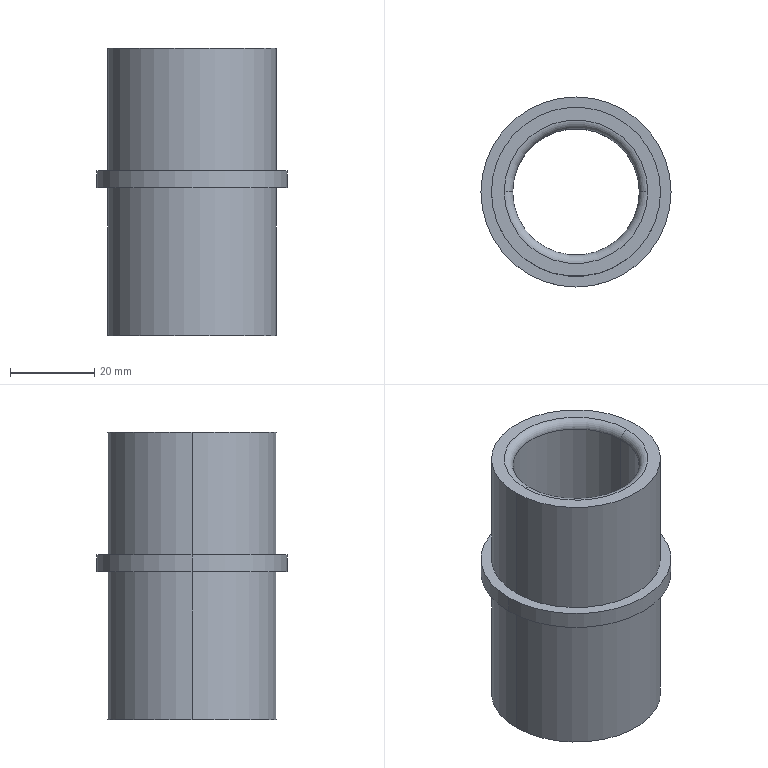Part | SolidWorks | features BaseBody 1 | 1 solid | 16 faces | box 45 x 45 x 68 mm | volume 38554 mm3 | cylinder 8 | torus 4 | plane 4 | commonest cylinder face diameters 40 x4 30 x2 45 x2
STEP:
#1=CARTESIAN_POINT('',(-288.,-175.,-311.5));
#2=VERTEX_POINT('',#1);
#3=CARTESIAN_POINT('',(-254.,-175.,-311.5));
#4=VERTEX_POINT('',#3);
#5=CARTESIAN_POINT('',(-271.,-175.,-311.5));
#6=DIRECTION('',(0.,0.,1.));
#7=DIRECTION('',(-1.,0.,0.));
#8=AXIS2_PLACEMENT_3D('',#5,#6,#7);
#9=CIRCLE('',#8,17.);
#10=EDGE_CURVE('',#2,#4,#9,.T.);
#11=ORIENTED_EDGE('',*,*,#10,.T.);
#12=CARTESIAN_POINT('',(-256.,-175.,-313.5));
#13=VERTEX_POINT('',#12);
#14=CARTESIAN_POINT('',(-254.,-175.,-313.5));
#15=DIRECTION('',(0.,-1.,0.));
#16=DIRECTION('',(1.,0.,0.));
#17=AXIS2_PLACEMENT_3D('',#14,#15,#16);
#18=CIRCLE('',#17,2.);
#19=EDGE_CURVE('',#4,#13,#18,.T.);
#20=ORIENTED_EDGE('',*,*,#19,.T.);
#21=CARTESIAN_POINT('',(-286.,-175.,-313.5));
#22=VERTEX_POINT('',#21);
#23=CARTESIAN_POINT('',(-271.,-175.,-313.5));
#24=DIRECTION('',(0.,0.,-1.));
#25=DIRECTION('',(-1.,0.,0.));
#26=AXIS2_PLACEMENT_3D('',#23,#24,#25);
#27=CIRCLE('',#26,15.);
#28=EDGE_CURVE('',#13,#22,#27,.T.);
#29=ORIENTED_EDGE('',*,*,#28,.T.);
#30=CARTESIAN_POINT('',(-288.,-175.,-313.5));
#31=DIRECTION('',(0.,1.,0.));
#32=DIRECTION('',(0.,0.,1.));
#33=AXIS2_PLACEMENT_3D('',#30,#31,#32);
#34=CIRCLE('',#33,2.);
#35=EDGE_CURVE('',#2,#22,#34,.T.);
#36=ORIENTED_EDGE('',*,*,#35,.F.);
#37=EDGE_LOOP('',(#11,#20,#29,#36));
#38=FACE_OUTER_BOUND('',#37,.T.);
#39=CARTESIAN_POINT('',(-271.,-175.,-313.5));
#40=DIRECTION('',(0.,0.,1.));
#41=DIRECTION('',(-1.,0.,0.));
#42=AXIS2_PLACEMENT_3D('',#39,#40,#41);
#43=TOROIDAL_SURFACE('',#42,17.,2.);
#44=ADVANCED_FACE('',(#38),#43,.T.);
#45=CARTESIAN_POINT('',(-251.,-175.,-311.5));
#46=VERTEX_POINT('',#45);
#47=CARTESIAN_POINT('',(-291.,-175.,-311.5));
#48=VERTEX_POINT('',#47);
#49=CARTESIAN_POINT('',(-271.,-175.,-311.5));
#50=DIRECTION('',(0.,0.,-1.));
#51=DIRECTION('',(-1.,0.,0.));
#52=AXIS2_PLACEMENT_3D('',#49,#50,#51);
#53=CIRCLE('',#52,20.);
#54=EDGE_CURVE('',#46,#48,#53,.T.);
#55=ORIENTED_EDGE('',*,*,#54,.T.);
#56=CARTESIAN_POINT('',(-291.,-175.,-340.5));
#57=VERTEX_POINT('',#56);
#58=CARTESIAN_POINT('',(-291.,-175.,-305.5));
#59=DIRECTION('',(0.,0.,-1.));
#60=VECTOR('',#59,1000.);
#61=LINE('',#58,#60);
#62=EDGE_CURVE('',#48,#57,#61,.T.);
#63=ORIENTED_EDGE('',*,*,#62,.T.);
#64=CARTESIAN_POINT('',(-251.,-175.,-340.5));
#65=VERTEX_POINT('',#64);
#66=CARTESIAN_POINT('',(-271.,-175.,-340.5));
#67=DIRECTION('',(0.,0.,1.));
#68=DIRECTION('',(1.,0.,0.));
#69=AXIS2_PLACEMENT_3D('',#66,#67,#68);
#70=CIRCLE('',#69,20.);
#71=EDGE_CURVE('',#57,#65,#70,.T.);
#72=ORIENTED_EDGE('',*,*,#71,.T.);
#73=CARTESIAN_POINT('',(-251.,-175.,-305.5));
#74=DIRECTION('',(0.,0.,-1.));
#75=VECTOR('',#74,1000.);
#76=LINE('',#73,#75);
#77=EDGE_CURVE('',#46,#65,#76,.T.);
#78=ORIENTED_EDGE('',*,*,#77,.F.);
#79=EDGE_LOOP('',(#55,#63,#72,#78));
#80=FACE_OUTER_BOUND('',#79,.T.);
#81=CARTESIAN_POINT('',(-271.,-175.,-305.5));
#82=DIRECTION('',(0.,0.,-1.));
#83=DIRECTION('',(1.,0.,0.));
#84=AXIS2_PLACEMENT_3D('',#81,#82,#83);
#85=CYLINDRICAL_SURFACE('',#84,20.);
#86=ADVANCED_FACE('',(#80),#85,.T.);
#87=CARTESIAN_POINT('',(-293.5,-175.,-340.5));
#88=VERTEX_POINT('',#87);
#89=CARTESIAN_POINT('',(-248.5,-175.,-340.5));
#90=VERTEX_POINT('',#89);
#91=CARTESIAN_POINT('',(-271.,-175.,-340.5));
#92=DIRECTION('',(0.,0.,1.));
#93=DIRECTION('',(1.,0.,0.));
#94=AXIS2_PLACEMENT_3D('',#91,#92,#93);
#95=CIRCLE('',#94,22.5);
#96=EDGE_CURVE('',#88,#90,#95,.T.);
#97=ORIENTED_EDGE('',*,*,#96,.F.);
#98=CARTESIAN_POINT('',(-293.5,-175.,-344.5));
#99=VERTEX_POINT('',#98);
#100=CARTESIAN_POINT('',(-293.5,-175.,-305.5));
#101=DIRECTION('',(0.,0.,-1.));
#102=VECTOR('',#101,1000.);
#103=LINE('',#100,#102);
#104=EDGE_CURVE('',#88,#99,#103,.T.);
#105=ORIENTED_EDGE('',*,*,#104,.T.);
#106=CARTESIAN_POINT('',(-248.5,-175.,-344.5));
#107=VERTEX_POINT('',#106);
#108=CARTESIAN_POINT('',(-271.,-175.,-344.5));
#109=DIRECTION('',(0.,0.,1.));
#110=DIRECTION('',(1.,0.,0.));
#111=AXIS2_PLACEMENT_3D('',#108,#109,#110);
#112=CIRCLE('',#111,22.5);
#113=EDGE_CURVE('',#99,#107,#112,.T.);
#114=ORIENTED_EDGE('',*,*,#113,.T.);
#115=CARTESIAN_POINT('',(-248.5,-175.,-305.5));
#116=DIRECTION('',(0.,0.,-1.));
#117=VECTOR('',#116,1000.);
#118=LINE('',#115,#117);
#119=EDGE_CURVE('',#90,#107,#118,.T.);
#120=ORIENTED_EDGE('',*,*,#119,.F.);
#121=EDGE_LOOP('',(#97,#105,#114,#120));
#122=FACE_OUTER_BOUND('',#121,.T.);
#123=CARTESIAN_POINT('',(-271.,-175.,-305.5));
#124=DIRECTION('',(0.,0.,-1.));
#125=DIRECTION('',(1.,0.,0.));
#126=AXIS2_PLACEMENT_3D('',#123,#124,#125);
#127=CYLINDRICAL_SURFACE('',#126,22.5);
#128=ADVANCED_FACE('',(#122),#127,.T.);
#129=CARTESIAN_POINT('',(-291.,-175.,-344.5));
#130=VERTEX_POINT('',#129);
#131=CARTESIAN_POINT('',(-251.,-175.,-344.5));
#132=VERTEX_POINT('',#131);
#133=CARTESIAN_POINT('',(-271.,-175.,-344.5));
#134=DIRECTION('',(0.,0.,1.));
#135=DIRECTION('',(1.,0.,0.));
#136=AXIS2_PLACEMENT_3D('',#133,#134,#135);
#137=CIRCLE('',#136,20.);
#138=EDGE_CURVE('',#130,#132,#137,.T.);
#139=ORIENTED_EDGE('',*,*,#138,.F.);
#140=CARTESIAN_POINT('',(-291.,-175.,-379.5));
#141=VERTEX_POINT('',#140);
#142=CARTESIAN_POINT('',(-291.,-175.,-305.5));
#143=DIRECTION('',(0.,0.,-1.));
#144=VECTOR('',#143,1000.);
#145=LINE('',#142,#144);
#146=EDGE_CURVE('',#130,#141,#145,.T.);
#147=ORIENTED_EDGE('',*,*,#146,.T.);
#148=CARTESIAN_POINT('',(-251.,-175.,-379.5));
#149=VERTEX_POINT('',#148);
#150=CARTESIAN_POINT('',(-271.,-175.,-379.5));
#151=DIRECTION('',(0.,0.,-1.));
#152=DIRECTION('',(-1.,0.,0.));
#153=AXIS2_PLACEMENT_3D('',#150,#151,#152);
#154=CIRCLE('',#153,20.);
#155=EDGE_CURVE('',#149,#141,#154,.T.);
#156=ORIENTED_EDGE('',*,*,#155,.F.);
#157=CARTESIAN_POINT('',(-251.,-175.,-305.5));
#158=DIRECTION('',(0.,0.,-1.));
#159=VECTOR('',#158,1000.);
#160=LINE('',#157,#159);
#161=EDGE_CURVE('',#132,#149,#160,.T.);
#162=ORIENTED_EDGE('',*,*,#161,.F.);
#163=EDGE_LOOP('',(#139,#147,#156,#162));
#164=FACE_OUTER_BOUND('',#163,.T.);
#165=CARTESIAN_POINT('',(-271.,-175.,-305.5));
#166=DIRECTION('',(0.,0.,-1.));
#167=DIRECTION('',(1.,0.,0.));
#168=AXIS2_PLACEMENT_3D('',#165,#166,#167);
#169=CYLINDRICAL_SURFACE('',#168,20.);
#170=ADVANCED_FACE('',(#164),#169,.T.);
#171=CARTESIAN_POINT('',(-271.,-175.,-313.5));
#172=DIRECTION('',(0.,0.,-1.));
#173=DIRECTION('',(-1.,0.,0.));
#174=AXIS2_PLACEMENT_3D('',#171,#172,#173);
#175=CIRCLE('',#174,15.);
#176=EDGE_CURVE('',#22,#13,#175,.T.);
#177=ORIENTED_EDGE('',*,*,#176,.F.);
#178=CARTESIAN_POINT('',(-286.,-175.,-377.5));
#179=VERTEX_POINT('',#178);
#180=CARTESIAN_POINT('',(-286.,-175.,-305.5));
#181=DIRECTION('',(0.,0.,-1.));
#182=VECTOR('',#181,1000.);
#183=LINE('',#180,#182);
#184=EDGE_CURVE('',#22,#179,#183,.T.);
#185=ORIENTED_EDGE('',*,*,#184,.T.);
#186=CARTESIAN_POINT('',(-256.,-175.,-377.5));
#187=VERTEX_POINT('',#186);
#188=CARTESIAN_POINT('',(-271.,-175.,-377.5));
#189=DIRECTION('',(0.,0.,1.));
#190=DIRECTION('',(-1.,0.,0.));
#191=AXIS2_PLACEMENT_3D('',#188,#189,#190);
#192=CIRCLE('',#191,15.);
#193=EDGE_CURVE('',#187,#179,#192,.T.);
#194=ORIENTED_EDGE('',*,*,#193,.F.);
#195=CARTESIAN_POINT('',(-256.,-175.,-305.5));
#196=DIRECTION('',(0.,0.,-1.));
#197=VECTOR('',#196,1000.);
#198=LINE('',#195,#197);
#199=EDGE_CURVE('',#13,#187,#198,.T.);
#200=ORIENTED_EDGE('',*,*,#199,.F.);
#201=EDGE_LOOP('',(#177,#185,#194,#200));
#202=FACE_OUTER_BOUND('',#201,.T.);
#203=CARTESIAN_POINT('',(-271.,-175.,-305.5));
#204=DIRECTION('',(0.,0.,-1.));
#205=DIRECTION('',(1.,0.,0.));
#206=AXIS2_PLACEMENT_3D('',#203,#204,#205);
#207=CYLINDRICAL_SURFACE('',#206,15.);
#208=ADVANCED_FACE('',(#202),#207,.F.);
#209=CARTESIAN_POINT('',(-271.,-175.,-377.5));
#210=DIRECTION('',(0.,0.,1.));
#211=DIRECTION('',(-1.,0.,0.));
#212=AXIS2_PLACEMENT_3D('',#209,#210,#211);
#213=CIRCLE('',#212,15.);
#214=EDGE_CURVE('',#179,#187,#213,.T.);
#215=ORIENTED_EDGE('',*,*,#214,.T.);
#216=CARTESIAN_POINT('',(-254.,-175.,-379.5));
#217=VERTEX_POINT('',#216);
#218=CARTESIAN_POINT('',(-254.,-175.,-377.5));
#219=DIRECTION('',(0.,-1.,0.));
#220=DIRECTION('',(1.,0.,0.));
#221=AXIS2_PLACEMENT_3D('',#218,#219,#220);
#222=CIRCLE('',#221,2.);
#223=EDGE_CURVE('',#187,#217,#222,.T.);
#224=ORIENTED_EDGE('',*,*,#223,.T.);
#225=CARTESIAN_POINT('',(-288.,-175.,-379.5));
#226=VERTEX_POINT('',#225);
#227=CARTESIAN_POINT('',(-271.,-175.,-379.5));
#228=DIRECTION('',(0.,0.,-1.));
#229=DIRECTION('',(-1.,0.,0.));
#230=AXIS2_PLACEMENT_3D('',#227,#228,#229);
#231=CIRCLE('',#230,17.);
#232=EDGE_CURVE('',#217,#226,#231,.T.);
#233=ORIENTED_EDGE('',*,*,#232,.T.);
#234=CARTESIAN_POINT('',(-288.,-175.,-377.5));
#235=DIRECTION('',(0.,1.,0.));
#236=DIRECTION('',(0.,0.,1.));
#237=AXIS2_PLACEMENT_3D('',#234,#235,#236);
#238=CIRCLE('',#237,2.);
#239=EDGE_CURVE('',#179,#226,#238,.T.);
#240=ORIENTED_EDGE('',*,*,#239,.F.);
#241=EDGE_LOOP('',(#215,#224,#233,#240));
#242=FACE_OUTER_BOUND('',#241,.T.);
#243=CARTESIAN_POINT('',(-271.,-175.,-377.5));
#244=DIRECTION('',(0.,0.,1.));
#245=DIRECTION('',(-1.,0.,0.));
#246=AXIS2_PLACEMENT_3D('',#243,#244,#245);
#247=TOROIDAL_SURFACE('',#246,17.,2.);
#248=ADVANCED_FACE('',(#242),#247,.T.);
#249=ORIENTED_EDGE('',*,*,#223,.F.);
#250=ORIENTED_EDGE('',*,*,#193,.T.);
#251=ORIENTED_EDGE('',*,*,#239,.T.);
#252=CARTESIAN_POINT('',(-271.,-175.,-379.5));
#253=DIRECTION('',(0.,0.,-1.));
#254=DIRECTION('',(-1.,0.,0.));
#255=AXIS2_PLACEMENT_3D('',#252,#253,#254);
#256=CIRCLE('',#255,17.);
#257=EDGE_CURVE('',#226,#217,#256,.T.);
#258=ORIENTED_EDGE('',*,*,#257,.T.);
#259=EDGE_LOOP('',(#249,#250,#251,#258));
#260=FACE_OUTER_BOUND('',#259,.T.);
#261=CARTESIAN_POINT('',(-271.,-175.,-377.5));
#262=DIRECTION('',(0.,0.,1.));
#263=DIRECTION('',(-1.,0.,0.));
#264=AXIS2_PLACEMENT_3D('',#261,#262,#263);
#265=TOROIDAL_SURFACE('',#264,17.,2.);
#266=ADVANCED_FACE('',(#260),#265,.T.);
#267=ORIENTED_EDGE('',*,*,#184,.F.);
#268=ORIENTED_EDGE('',*,*,#28,.F.);
#269=ORIENTED_EDGE('',*,*,#199,.T.);
#270=ORIENTED_EDGE('',*,*,#214,.F.);
#271=EDGE_LOOP('',(#267,#268,#269,#270));
#272=FACE_OUTER_BOUND('',#271,.T.);
#273=CARTESIAN_POINT('',(-271.,-175.,-305.5));
#274=DIRECTION('',(0.,0.,-1.));
#275=DIRECTION('',(1.,0.,0.));
#276=AXIS2_PLACEMENT_3D('',#273,#274,#275);
#277=CYLINDRICAL_SURFACE('',#276,15.);
#278=ADVANCED_FACE('',(#272),#277,.F.);
#279=ORIENTED_EDGE('',*,*,#257,.F.);
#280=ORIENTED_EDGE('',*,*,#232,.F.);
#281=EDGE_LOOP('',(#279,#280));
#282=FACE_BOUND('',#281,.T.);
#283=ORIENTED_EDGE('',*,*,#155,.T.);
#284=CARTESIAN_POINT('',(-271.,-175.,-379.5));
#285=DIRECTION('',(0.,0.,-1.));
#286=DIRECTION('',(-1.,0.,0.));
#287=AXIS2_PLACEMENT_3D('',#284,#285,#286);
#288=CIRCLE('',#287,20.);
#289=EDGE_CURVE('',#141,#149,#288,.T.);
#290=ORIENTED_EDGE('',*,*,#289,.T.);
#291=EDGE_LOOP('',(#283,#290));
#292=FACE_OUTER_BOUND('',#291,.T.);
#293=CARTESIAN_POINT('',(-271.,-175.,-379.5));
#294=DIRECTION('',(0.,0.,1.));
#295=DIRECTION('',(-1.,0.,0.));
#296=AXIS2_PLACEMENT_3D('',#293,#294,#295);
#297=PLANE('',#296);
#298=ADVANCED_FACE('',(#282,#292),#297,.F.);
#299=ORIENTED_EDGE('',*,*,#146,.F.);
#300=CARTESIAN_POINT('',(-271.,-175.,-344.5));
#301=DIRECTION('',(0.,0.,1.));
#302=DIRECTION('',(1.,0.,0.));
#303=AXIS2_PLACEMENT_3D('',#300,#301,#302);
#304=CIRCLE('',#303,20.);
#305=EDGE_CURVE('',#132,#130,#304,.T.);
#306=ORIENTED_EDGE('',*,*,#305,.F.);
#307=ORIENTED_EDGE('',*,*,#161,.T.);
#308=ORIENTED_EDGE('',*,*,#289,.F.);
#309=EDGE_LOOP('',(#299,#306,#307,#308));
#310=FACE_OUTER_BOUND('',#309,.T.);
#311=CARTESIAN_POINT('',(-271.,-175.,-305.5));
#312=DIRECTION('',(0.,0.,-1.));
#313=DIRECTION('',(1.,0.,0.));
#314=AXIS2_PLACEMENT_3D('',#311,#312,#313);
#315=CYLINDRICAL_SURFACE('',#314,20.);
#316=ADVANCED_FACE('',(#310),#315,.T.);
#317=CARTESIAN_POINT('',(-271.,-175.,-344.5));
#318=DIRECTION('',(0.,0.,1.));
#319=DIRECTION('',(1.,0.,0.));
#320=AXIS2_PLACEMENT_3D('',#317,#318,#319);
#321=CIRCLE('',#320,22.5);
#322=EDGE_CURVE('',#107,#99,#321,.T.);
#323=ORIENTED_EDGE('',*,*,#322,.F.);
#324=ORIENTED_EDGE('',*,*,#113,.F.);
#325=EDGE_LOOP('',(#323,#324));
#326=FACE_OUTER_BOUND('',#325,.T.);
#327=ORIENTED_EDGE('',*,*,#305,.T.);
#328=ORIENTED_EDGE('',*,*,#138,.T.);
#329=EDGE_LOOP('',(#327,#328));
#330=FACE_BOUND('',#329,.T.);
#331=CARTESIAN_POINT('',(25.,-350.,-344.5));
#332=DIRECTION('',(0.,0.,-1.));
#333=DIRECTION('',(1.,0.,0.));
#334=AXIS2_PLACEMENT_3D('',#331,#332,#333);
#335=PLANE('',#334);
#336=ADVANCED_FACE('',(#326,#330),#335,.T.);
#337=CARTESIAN_POINT('',(-271.,-175.,-340.5));
#338=DIRECTION('',(0.,0.,1.));
#339=DIRECTION('',(1.,0.,0.));
#340=AXIS2_PLACEMENT_3D('',#337,#338,#339);
#341=CIRCLE('',#340,20.);
#342=EDGE_CURVE('',#65,#57,#341,.T.);
#343=ORIENTED_EDGE('',*,*,#342,.F.);
#344=ORIENTED_EDGE('',*,*,#71,.F.);
#345=EDGE_LOOP('',(#343,#344));
#346=FACE_BOUND('',#345,.T.);
#347=CARTESIAN_POINT('',(-271.,-175.,-340.5));
#348=DIRECTION('',(0.,0.,1.));
#349=DIRECTION('',(1.,0.,0.));
#350=AXIS2_PLACEMENT_3D('',#347,#348,#349);
#351=CIRCLE('',#350,22.5);
#352=EDGE_CURVE('',#90,#88,#351,.T.);
#353=ORIENTED_EDGE('',*,*,#352,.T.);
#354=ORIENTED_EDGE('',*,*,#96,.T.);
#355=EDGE_LOOP('',(#353,#354));
#356=FACE_OUTER_BOUND('',#355,.T.);
#357=CARTESIAN_POINT('',(25.,-350.,-340.5));
#358=DIRECTION('',(0.,0.,-1.));
#359=DIRECTION('',(1.,0.,0.));
#360=AXIS2_PLACEMENT_3D('',#357,#358,#359);
#361=PLANE('',#360);
#362=ADVANCED_FACE('',(#346,#356),#361,.F.);
#363=ORIENTED_EDGE('',*,*,#104,.F.);
#364=ORIENTED_EDGE('',*,*,#352,.F.);
#365=ORIENTED_EDGE('',*,*,#119,.T.);
#366=ORIENTED_EDGE('',*,*,#322,.T.);
#367=EDGE_LOOP('',(#363,#364,#365,#366));
#368=FACE_OUTER_BOUND('',#367,.T.);
#369=CARTESIAN_POINT('',(-271.,-175.,-305.5));
#370=DIRECTION('',(0.,0.,-1.));
#371=DIRECTION('',(1.,0.,0.));
#372=AXIS2_PLACEMENT_3D('',#369,#370,#371);
#373=CYLINDRICAL_SURFACE('',#372,22.5);
#374=ADVANCED_FACE('',(#368),#373,.T.);
#375=ORIENTED_EDGE('',*,*,#62,.F.);
#376=CARTESIAN_POINT('',(-271.,-175.,-311.5));
#377=DIRECTION('',(0.,0.,-1.));
#378=DIRECTION('',(-1.,0.,0.));
#379=AXIS2_PLACEMENT_3D('',#376,#377,#378);
#380=CIRCLE('',#379,20.);
#381=EDGE_CURVE('',#48,#46,#380,.T.);
#382=ORIENTED_EDGE('',*,*,#381,.T.);
#383=ORIENTED_EDGE('',*,*,#77,.T.);
#384=ORIENTED_EDGE('',*,*,#342,.T.);
#385=EDGE_LOOP('',(#375,#382,#383,#384));
#386=FACE_OUTER_BOUND('',#385,.T.);
#387=CARTESIAN_POINT('',(-271.,-175.,-305.5));
#388=DIRECTION('',(0.,0.,-1.));
#389=DIRECTION('',(1.,0.,0.));
#390=AXIS2_PLACEMENT_3D('',#387,#388,#389);
#391=CYLINDRICAL_SURFACE('',#390,20.);
#392=ADVANCED_FACE('',(#386),#391,.T.);
#393=ORIENTED_EDGE('',*,*,#10,.F.);
#394=CARTESIAN_POINT('',(-271.,-175.,-311.5));
#395=DIRECTION('',(0.,0.,1.));
#396=DIRECTION('',(-1.,0.,0.));
#397=AXIS2_PLACEMENT_3D('',#394,#395,#396);
#398=CIRCLE('',#397,17.);
#399=EDGE_CURVE('',#4,#2,#398,.T.);
#400=ORIENTED_EDGE('',*,*,#399,.F.);
#401=EDGE_LOOP('',(#393,#400));
#402=FACE_BOUND('',#401,.T.);
#403=ORIENTED_EDGE('',*,*,#54,.F.);
#404=ORIENTED_EDGE('',*,*,#381,.F.);
#405=EDGE_LOOP('',(#403,#404));
#406=FACE_OUTER_BOUND('',#405,.T.);
#407=CARTESIAN_POINT('',(-271.,-175.,-311.5));
#408=DIRECTION('',(0.,0.,1.));
#409=DIRECTION('',(-1.,0.,0.));
#410=AXIS2_PLACEMENT_3D('',#407,#408,#409);
#411=PLANE('',#410);
#412=ADVANCED_FACE('',(#402,#406),#411,.T.);
#413=ORIENTED_EDGE('',*,*,#19,.F.);
#414=ORIENTED_EDGE('',*,*,#399,.T.);
#415=ORIENTED_EDGE('',*,*,#35,.T.);
#416=ORIENTED_EDGE('',*,*,#176,.T.);
#417=EDGE_LOOP('',(#413,#414,#415,#416));
#418=FACE_OUTER_BOUND('',#417,.T.);
#419=CARTESIAN_POINT('',(-271.,-175.,-313.5));
#420=DIRECTION('',(0.,0.,1.));
#421=DIRECTION('',(-1.,0.,0.));
#422=AXIS2_PLACEMENT_3D('',#419,#420,#421);
#423=TOROIDAL_SURFACE('',#422,17.,2.);
#424=ADVANCED_FACE('',(#418),#423,.T.);
#425=CLOSED_SHELL('',(#44,#86,#128,#170,#208,#248,#266,#278,#298,#316,#336,#362,#374,#392,#412,#424));
#426=MANIFOLD_SOLID_BREP('',#425);
#427=CARTESIAN_POINT('',(0.,0.,0.));
#428=DIRECTION('',(0.,0.,1.));
#429=DIRECTION('',(1.,0.,0.));
#430=AXIS2_PLACEMENT_3D('',#427,#428,#429);
#431=(LENGTH_UNIT()NAMED_UNIT(*)SI_UNIT(.MILLI.,.METRE.));
#432=UNCERTAINTY_MEASURE_WITH_UNIT(LENGTH_MEASURE(0.00001),#431,'','');
#433=(NAMED_UNIT(*)PLANE_ANGLE_UNIT()SI_UNIT($,.RADIAN.));
#434=(NAMED_UNIT(*)SI_UNIT($,.STERADIAN.)SOLID_ANGLE_UNIT());
#435=(GEOMETRIC_REPRESENTATION_CONTEXT(3)GLOBAL_UNCERTAINTY_ASSIGNED_CONTEXT((#432))GLOBAL_UNIT_ASSIGNED_CONTEXT((#431,#433,#434))REPRESENTATION_CONTEXT('',''));
#436=ADVANCED_BREP_SHAPE_REPRESENTATION('',(#426,#430),#435);